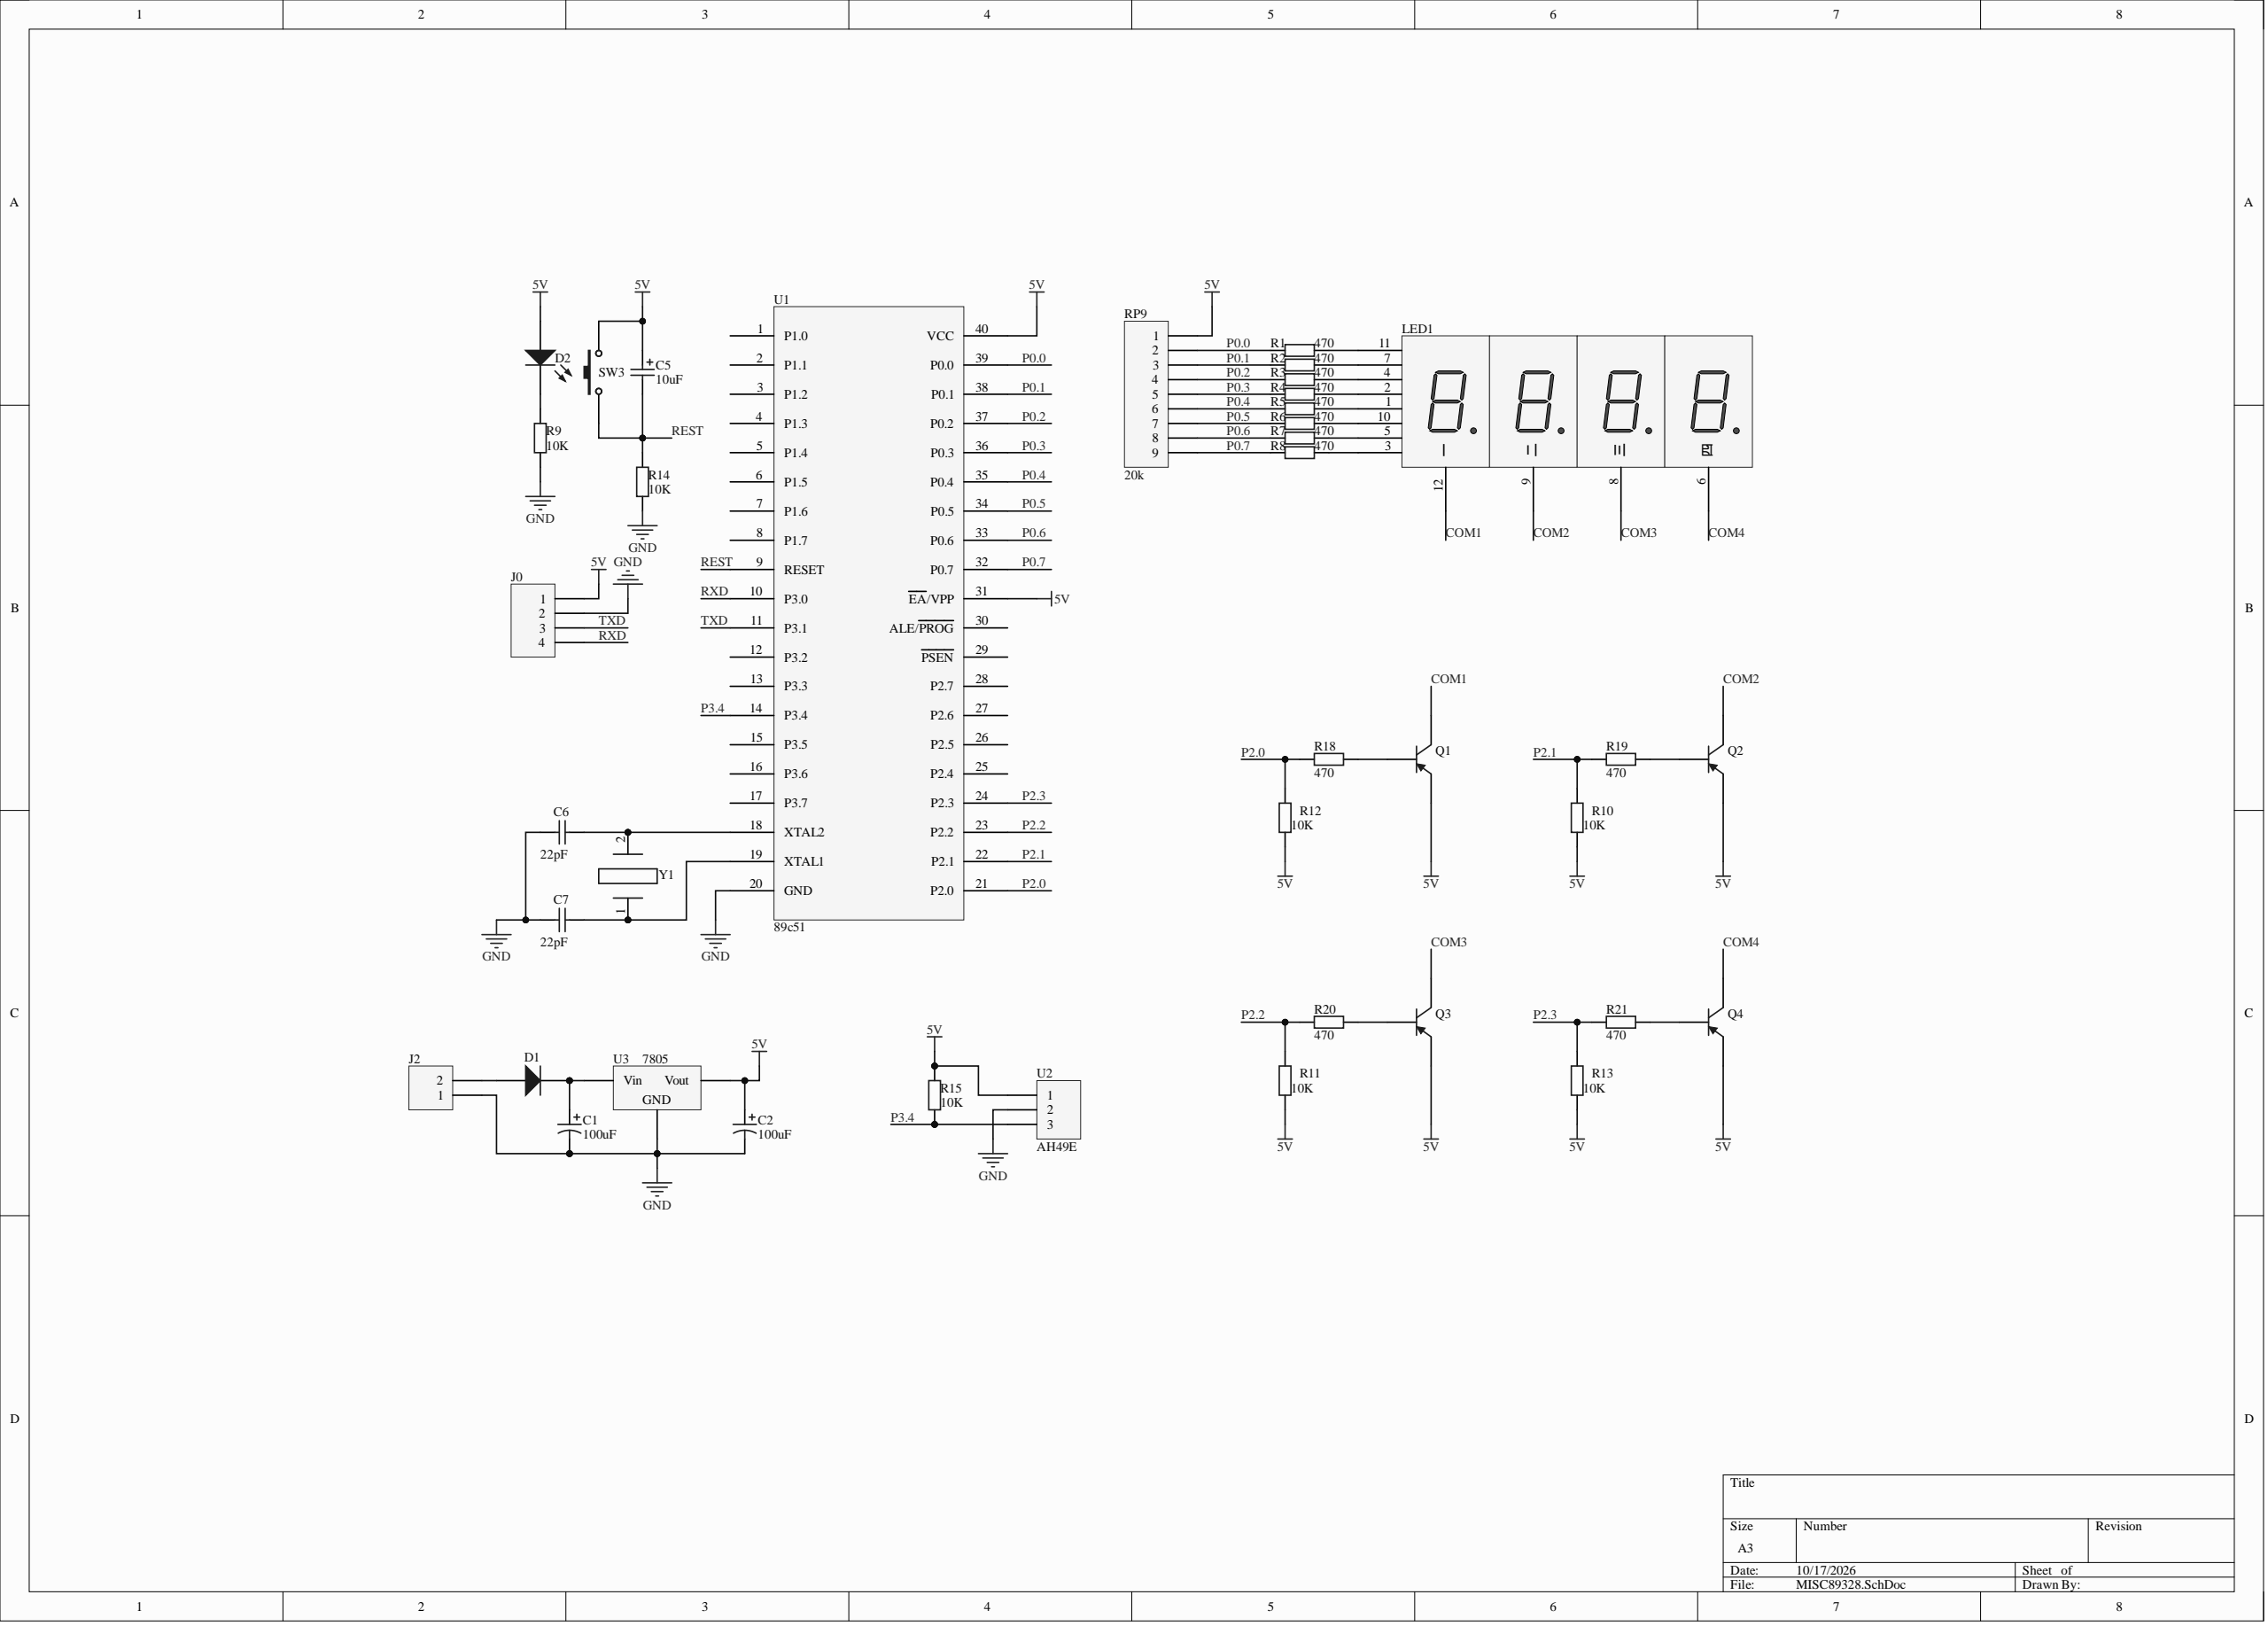Circuit board | Altium Designer | 39 parts | 39 nets
Bill of materials:
Comment,Description,Designator,Footprint,LibRef,Quantity
"100uF","Polarized Capacitor (Radial)","C1","RB7.6-15","Cap Pol1","1"
"Cap Pol1","Polarized Capacitor (Radial)","C2","RB7.6-15","Cap Pol1","1"
"Cap Pol2","Polarized Capacitor (Axial)","C5","POLAR0.8","Cap Pol2","1"
"Cap","Capacitor","C6, C7","RAD-0.3","Cap","2"
"Diode 1N914","High Conductance Fast Diode","D1","DO-35","Diode 1N914","1"
"LED0","Typical INFRARED GaAs LED","D2","LED-0","LED0","1"
"Header 4","Header, 4-Pin","J0","HDR1X4","Header 4","1"
"Header 2","Header, 2-Pin","J2","HDR1X2","Header 2","1"
"Dpy Red-CA","7.62 mm Black Surface HER 7-Segment Display: CA, RH DP","LED1","四位数码管","Dpy Red-CA","1"
"2N3906","PNP General Purpose Amplifier","Q1, Q2, Q3, Q4","TO-92A","2N3906","4"
"Res2","Resistor","R1, R2, R3, R4, R5, R6, R7, R8, R9, R10, R11, R12, R13, R14, R15, R18, R19, R20, R21","AXIAL-0.4","Res2","19"
"20k","Header, 9-Pin","RP9","HDR1X9","Header 9","1"
"SW-PB","Switch","SW3","SPST-2","SW-PB","1"
"89c51","","U1","89c51","Component_1","1"
"AH49E","Header, 3-Pin","U2","HDR1X3","Header 3","1"
"7805","Voltage Regulator","U3","PCBComponent_1","Volt Reg","1"
"Component_1","","Y1","LC-HC-49S","Component_1","1"
Netlist (Protel format):
[
C1
RB7.6-15
100uF



]
[
C2
RB7.6-15
Cap Pol1



]
[
C5
POLAR0.8
Cap Pol2



]
[
C6
RAD-0.3
Cap



]
[
C7
RAD-0.3
Cap



]
[
D1
DO-35
Diode 1N914



]
[
D2
LED-0
LED0



]
[
J0
HDR1X4
Header 4



]
[
J2
HDR1X2
Header 2



]
[
LED1
四位数码管
Dpy Red-CA



]
[
Q1
TO-92A
2N3906



]
[
Q2
TO-92A
2N3906



]
[
Q3
TO-92A
2N3906



]
[
Q4
TO-92A
2N3906



]
[
R1
AXIAL-0.4
Res2



]
[
R2
AXIAL-0.4
Res2



]
[
R3
AXIAL-0.4
Res2



]
[
R4
AXIAL-0.4
Res2



]
[
R5
AXIAL-0.4
Res2



]
[
R6
AXIAL-0.4
Res2



]
[
R7
AXIAL-0.4
Res2



]
[
R8
AXIAL-0.4
Res2



]
[
R9
AXIAL-0.4
Res2



]
[
R10
AXIAL-0.4
Res2



]
[
R11
AXIAL-0.4
Res2



]
[
R12
AXIAL-0.4
Res2



]
[
R13
AXIAL-0.4
Res2



]
[
R14
AXIAL-0.4
Res2



]
[
R15
AXIAL-0.4
Res2



]
[
R18
AXIAL-0.4
Res2



]
[
R19
AXIAL-0.4
Res2



]
[
R20
AXIAL-0.4
Res2



]
[
R21
AXIAL-0.4
Res2



]
[
RP9
HDR1X9
20k



]
[
SW3
SPST-2
SW-PB



]
[
U1
89c51
89c51



]
[
U2
HDR1X3
AH49E



]
[
U3
PCBComponent_1
7805



]
[
Y1
LC-HC-49S
Component_1



]
(
TXD
J0-3
U1-11
)
(
RXD
J0-4
U1-10
)
(
REST
C5-2
R14-1
SW3-1
U1-9
)
(
P3.4
R15-1
U1-14
U2-3
)
(
P2.3
R13-2
R21-2
U1-24
)
(
P2.2
R11-2
R20-2
U1-23
)
(
P2.1
R10-2
R19-2
U1-22
)
(
P2.0
R12-2
R18-2
U1-21
)
(
P0.7
R8-1
RP9-9
U1-32
)
(
P0.6
R7-1
RP9-8
U1-33
)
(
P0.5
R6-1
RP9-7
U1-34
)
(
P0.4
R5-1
RP9-6
U1-35
)
(
P0.3
R4-1
RP9-5
U1-36
)
(
P0.2
R3-1
RP9-4
U1-37
)
(
P0.1
R2-1
RP9-3
U1-38
)
(
P0.0
R1-1
RP9-2
U1-39
)
(
NetQ4_2
Q4-2
R21-1
)
(
NetQ3_2
Q3-2
R20-1
)
(
NetQ2_2
Q2-2
R19-1
)
(
NetQ1_2
Q1-2
R18-1
)
(
NetLED1_11
LED1-11
R1-2
)
(
NetLED1_10
LED1-10
R6-2
)
(
NetLED1_7
LED1-7
R2-2
)
(
NetLED1_5
LED1-5
R7-2
)
(
NetLED1_4
LED1-4
R3-2
)
(
NetLED1_3
LED1-3
R8-2
)
(
NetLED1_2
LED1-2
R4-2
)
(
NetLED1_1
LED1-1
R5-2
)
(
NetD2_2
D2-2
R9-1
)
(
NetD1_1
D1-1
J2-2
)
(
NetC7_1
C7-1
U1-19
Y1-1
)
(
NetC6_1
C6-1
U1-18
Y1-2
)
(
NetC1_1
C1-1
D1-2
U3-1
)
(
GND
C1-2
C2-2
C6-2
C7-2
J0-2
J2-1
R9-2
R14-2
U1-20
U2-2
U3-2
)
(
COM4
LED1-6
Q4-3
)
(
COM3
LED1-8
Q3-3
)
(
COM2
LED1-9
Q2-3
)
(
COM1
LED1-12
Q1-3
)
(
5V
C2-1
C5-1
D2-1
J0-1
Q1-1
Q2-1
Q3-1
Q4-1
R10-1
R11-1
R12-1
R13-1
R15-2
RP9-1
SW3-2
U1-31
U1-40
U2-1
U3-3
)